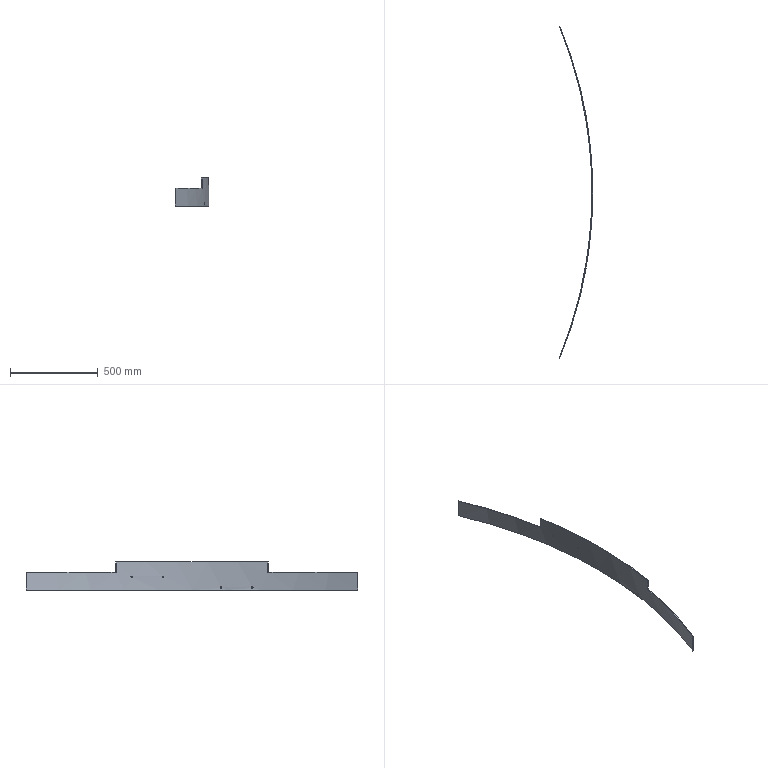Part | STEP file | 19-Side baffle 1 | 1 solid | 18 faces | box 190.691 x 1891 x 160 mm | volume 983357 mm3 | spline 8 | plane 8 | cylinder 2 | commonest cylinder face diameters 4960 x1 4968 x1